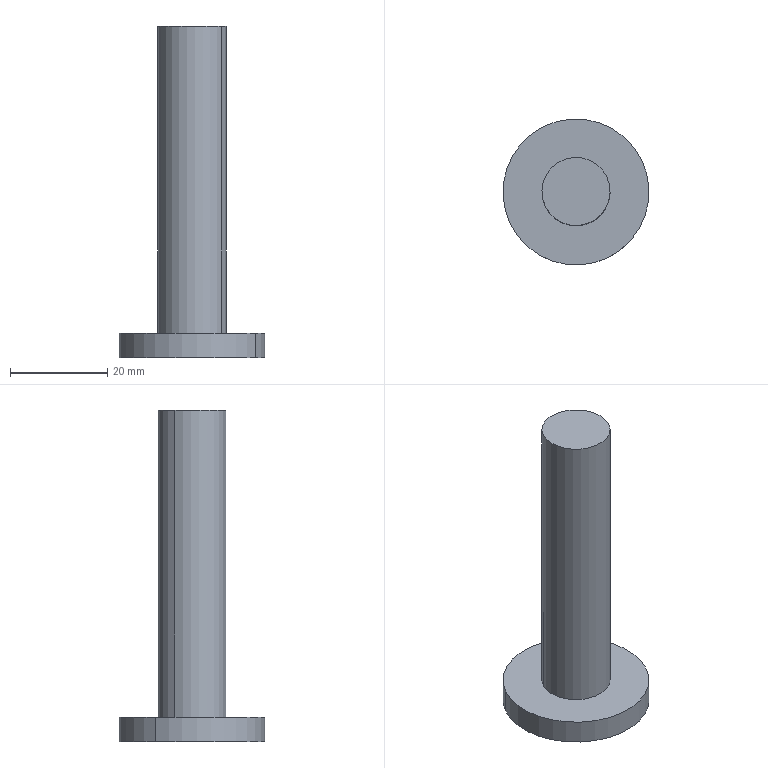Part | SolidWorks | features BaseBody 1 | 1 solid | 7 faces | box 30 x 30 x 68 mm | volume 13232 mm3 | cylinder 4 | plane 3 | commonest cylinder face diameters 14 x2 30 x2
STEP:
#1=CARTESIAN_POINT('',(475.1,-26.347,-429.));
#2=VERTEX_POINT('',#1);
#3=CARTESIAN_POINT('',(487.224,-33.347,-429.));
#4=VERTEX_POINT('',#3);
#5=CARTESIAN_POINT('',(481.162,-29.847,-429.));
#6=DIRECTION('',(0.,0.,1.));
#7=DIRECTION('',(-0.866,0.5,0.));
#8=AXIS2_PLACEMENT_3D('',#5,#6,#7);
#9=CIRCLE('',#8,7.);
#10=EDGE_CURVE('',#2,#4,#9,.T.);
#11=ORIENTED_EDGE('',*,*,#10,.F.);
#12=CARTESIAN_POINT('',(475.1,-26.347,-492.));
#13=VERTEX_POINT('',#12);
#14=CARTESIAN_POINT('',(475.1,-26.347,-429.));
#15=DIRECTION('',(0.,0.,-1.));
#16=VECTOR('',#15,1000.);
#17=LINE('',#14,#16);
#18=EDGE_CURVE('',#2,#13,#17,.T.);
#19=ORIENTED_EDGE('',*,*,#18,.T.);
#20=CARTESIAN_POINT('',(487.224,-33.347,-492.));
#21=VERTEX_POINT('',#20);
#22=CARTESIAN_POINT('',(481.162,-29.847,-492.));
#23=DIRECTION('',(0.,0.,1.));
#24=DIRECTION('',(-0.866,0.5,0.));
#25=AXIS2_PLACEMENT_3D('',#22,#23,#24);
#26=CIRCLE('',#25,7.);
#27=EDGE_CURVE('',#13,#21,#26,.T.);
#28=ORIENTED_EDGE('',*,*,#27,.T.);
#29=CARTESIAN_POINT('',(487.224,-33.347,-429.));
#30=DIRECTION('',(0.,0.,-1.));
#31=VECTOR('',#30,1000.);
#32=LINE('',#29,#31);
#33=EDGE_CURVE('',#4,#21,#32,.T.);
#34=ORIENTED_EDGE('',*,*,#33,.F.);
#35=EDGE_LOOP('',(#11,#19,#28,#34));
#36=FACE_OUTER_BOUND('',#35,.T.);
#37=CARTESIAN_POINT('',(481.162,-29.847,-429.));
#38=DIRECTION('',(0.,0.,-1.));
#39=DIRECTION('',(0.866,-0.5,0.));
#40=AXIS2_PLACEMENT_3D('',#37,#38,#39);
#41=CYLINDRICAL_SURFACE('',#40,7.);
#42=ADVANCED_FACE('',(#36),#41,.T.);
#43=CARTESIAN_POINT('',(468.172,-22.347,-492.));
#44=VERTEX_POINT('',#43);
#45=CARTESIAN_POINT('',(494.153,-37.347,-492.));
#46=VERTEX_POINT('',#45);
#47=CARTESIAN_POINT('',(481.162,-29.847,-492.));
#48=DIRECTION('',(0.,0.,1.));
#49=DIRECTION('',(-0.866,0.5,0.));
#50=AXIS2_PLACEMENT_3D('',#47,#48,#49);
#51=CIRCLE('',#50,15.);
#52=EDGE_CURVE('',#44,#46,#51,.T.);
#53=ORIENTED_EDGE('',*,*,#52,.F.);
#54=CARTESIAN_POINT('',(468.172,-22.347,-497.));
#55=VERTEX_POINT('',#54);
#56=CARTESIAN_POINT('',(468.172,-22.347,-492.));
#57=DIRECTION('',(0.,0.,-1.));
#58=VECTOR('',#57,1000.);
#59=LINE('',#56,#58);
#60=EDGE_CURVE('',#44,#55,#59,.T.);
#61=ORIENTED_EDGE('',*,*,#60,.T.);
#62=CARTESIAN_POINT('',(494.153,-37.347,-497.));
#63=VERTEX_POINT('',#62);
#64=CARTESIAN_POINT('',(481.162,-29.847,-497.));
#65=DIRECTION('',(0.,0.,1.));
#66=DIRECTION('',(-0.866,0.5,0.));
#67=AXIS2_PLACEMENT_3D('',#64,#65,#66);
#68=CIRCLE('',#67,15.);
#69=EDGE_CURVE('',#55,#63,#68,.T.);
#70=ORIENTED_EDGE('',*,*,#69,.T.);
#71=CARTESIAN_POINT('',(494.153,-37.347,-492.));
#72=DIRECTION('',(0.,0.,-1.));
#73=VECTOR('',#72,1000.);
#74=LINE('',#71,#73);
#75=EDGE_CURVE('',#46,#63,#74,.T.);
#76=ORIENTED_EDGE('',*,*,#75,.F.);
#77=EDGE_LOOP('',(#53,#61,#70,#76));
#78=FACE_OUTER_BOUND('',#77,.T.);
#79=CARTESIAN_POINT('',(481.162,-29.847,-492.));
#80=DIRECTION('',(0.,0.,-1.));
#81=DIRECTION('',(0.866,-0.5,0.));
#82=AXIS2_PLACEMENT_3D('',#79,#80,#81);
#83=CYLINDRICAL_SURFACE('',#82,15.);
#84=ADVANCED_FACE('',(#78),#83,.T.);
#85=CARTESIAN_POINT('',(481.162,-29.847,-492.));
#86=DIRECTION('',(0.,0.,1.));
#87=DIRECTION('',(-0.866,0.5,0.));
#88=AXIS2_PLACEMENT_3D('',#85,#86,#87);
#89=CIRCLE('',#88,15.);
#90=EDGE_CURVE('',#46,#44,#89,.T.);
#91=ORIENTED_EDGE('',*,*,#90,.T.);
#92=ORIENTED_EDGE('',*,*,#52,.T.);
#93=EDGE_LOOP('',(#91,#92));
#94=FACE_OUTER_BOUND('',#93,.T.);
#95=CARTESIAN_POINT('',(481.162,-29.847,-492.));
#96=DIRECTION('',(0.,0.,1.));
#97=DIRECTION('',(-0.866,0.5,0.));
#98=AXIS2_PLACEMENT_3D('',#95,#96,#97);
#99=CIRCLE('',#98,7.);
#100=EDGE_CURVE('',#21,#13,#99,.T.);
#101=ORIENTED_EDGE('',*,*,#100,.F.);
#102=ORIENTED_EDGE('',*,*,#27,.F.);
#103=EDGE_LOOP('',(#101,#102));
#104=FACE_BOUND('',#103,.T.);
#105=CARTESIAN_POINT('',(481.162,-29.847,-492.));
#106=DIRECTION('',(0.,0.,1.));
#107=DIRECTION('',(-0.866,0.5,0.));
#108=AXIS2_PLACEMENT_3D('',#105,#106,#107);
#109=PLANE('',#108);
#110=ADVANCED_FACE('',(#94,#104),#109,.T.);
#111=ORIENTED_EDGE('',*,*,#60,.F.);
#112=ORIENTED_EDGE('',*,*,#90,.F.);
#113=ORIENTED_EDGE('',*,*,#75,.T.);
#114=CARTESIAN_POINT('',(481.162,-29.847,-497.));
#115=DIRECTION('',(0.,0.,1.));
#116=DIRECTION('',(-0.866,0.5,0.));
#117=AXIS2_PLACEMENT_3D('',#114,#115,#116);
#118=CIRCLE('',#117,15.);
#119=EDGE_CURVE('',#63,#55,#118,.T.);
#120=ORIENTED_EDGE('',*,*,#119,.T.);
#121=EDGE_LOOP('',(#111,#112,#113,#120));
#122=FACE_OUTER_BOUND('',#121,.T.);
#123=CARTESIAN_POINT('',(481.162,-29.847,-492.));
#124=DIRECTION('',(0.,0.,-1.));
#125=DIRECTION('',(0.866,-0.5,0.));
#126=AXIS2_PLACEMENT_3D('',#123,#124,#125);
#127=CYLINDRICAL_SURFACE('',#126,15.);
#128=ADVANCED_FACE('',(#122),#127,.T.);
#129=ORIENTED_EDGE('',*,*,#119,.F.);
#130=ORIENTED_EDGE('',*,*,#69,.F.);
#131=EDGE_LOOP('',(#129,#130));
#132=FACE_OUTER_BOUND('',#131,.T.);
#133=CARTESIAN_POINT('',(481.162,-29.847,-497.));
#134=DIRECTION('',(0.,0.,1.));
#135=DIRECTION('',(-0.866,0.5,0.));
#136=AXIS2_PLACEMENT_3D('',#133,#134,#135);
#137=PLANE('',#136);
#138=ADVANCED_FACE('',(#132),#137,.F.);
#139=ORIENTED_EDGE('',*,*,#18,.F.);
#140=CARTESIAN_POINT('',(481.162,-29.847,-429.));
#141=DIRECTION('',(0.,0.,1.));
#142=DIRECTION('',(-0.866,0.5,0.));
#143=AXIS2_PLACEMENT_3D('',#140,#141,#142);
#144=CIRCLE('',#143,7.);
#145=EDGE_CURVE('',#4,#2,#144,.T.);
#146=ORIENTED_EDGE('',*,*,#145,.F.);
#147=ORIENTED_EDGE('',*,*,#33,.T.);
#148=ORIENTED_EDGE('',*,*,#100,.T.);
#149=EDGE_LOOP('',(#139,#146,#147,#148));
#150=FACE_OUTER_BOUND('',#149,.T.);
#151=CARTESIAN_POINT('',(481.162,-29.847,-429.));
#152=DIRECTION('',(0.,0.,-1.));
#153=DIRECTION('',(0.866,-0.5,0.));
#154=AXIS2_PLACEMENT_3D('',#151,#152,#153);
#155=CYLINDRICAL_SURFACE('',#154,7.);
#156=ADVANCED_FACE('',(#150),#155,.T.);
#157=ORIENTED_EDGE('',*,*,#145,.T.);
#158=ORIENTED_EDGE('',*,*,#10,.T.);
#159=EDGE_LOOP('',(#157,#158));
#160=FACE_OUTER_BOUND('',#159,.T.);
#161=CARTESIAN_POINT('',(481.162,-29.847,-429.));
#162=DIRECTION('',(0.,0.,1.));
#163=DIRECTION('',(-0.866,0.5,0.));
#164=AXIS2_PLACEMENT_3D('',#161,#162,#163);
#165=PLANE('',#164);
#166=ADVANCED_FACE('',(#160),#165,.T.);
#167=CLOSED_SHELL('',(#42,#84,#110,#128,#138,#156,#166));
#168=MANIFOLD_SOLID_BREP('',#167);
#169=CARTESIAN_POINT('',(0.,0.,0.));
#170=DIRECTION('',(0.,0.,1.));
#171=DIRECTION('',(1.,0.,0.));
#172=AXIS2_PLACEMENT_3D('',#169,#170,#171);
#173=(LENGTH_UNIT()NAMED_UNIT(*)SI_UNIT(.MILLI.,.METRE.));
#174=UNCERTAINTY_MEASURE_WITH_UNIT(LENGTH_MEASURE(0.00001),#173,'','');
#175=(NAMED_UNIT(*)PLANE_ANGLE_UNIT()SI_UNIT($,.RADIAN.));
#176=(NAMED_UNIT(*)SI_UNIT($,.STERADIAN.)SOLID_ANGLE_UNIT());
#177=(GEOMETRIC_REPRESENTATION_CONTEXT(3)GLOBAL_UNCERTAINTY_ASSIGNED_CONTEXT((#174))GLOBAL_UNIT_ASSIGNED_CONTEXT((#173,#175,#176))REPRESENTATION_CONTEXT('',''));
#178=ADVANCED_BREP_SHAPE_REPRESENTATION('',(#168,#172),#177);